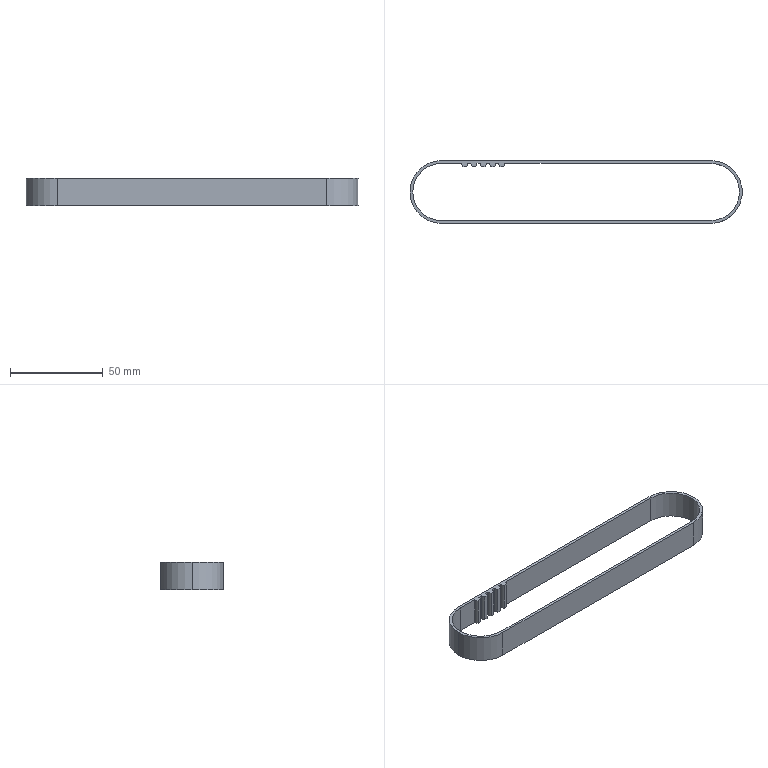Part | STEP file | 1 solid | 32 faces | box 178.871 x 33.871 x 15 mm | volume 9222 mm3 | cylinder 16 | plane 16 | commonest cylinder face diameters 6.5 x10 30.871 x3 33.871 x3